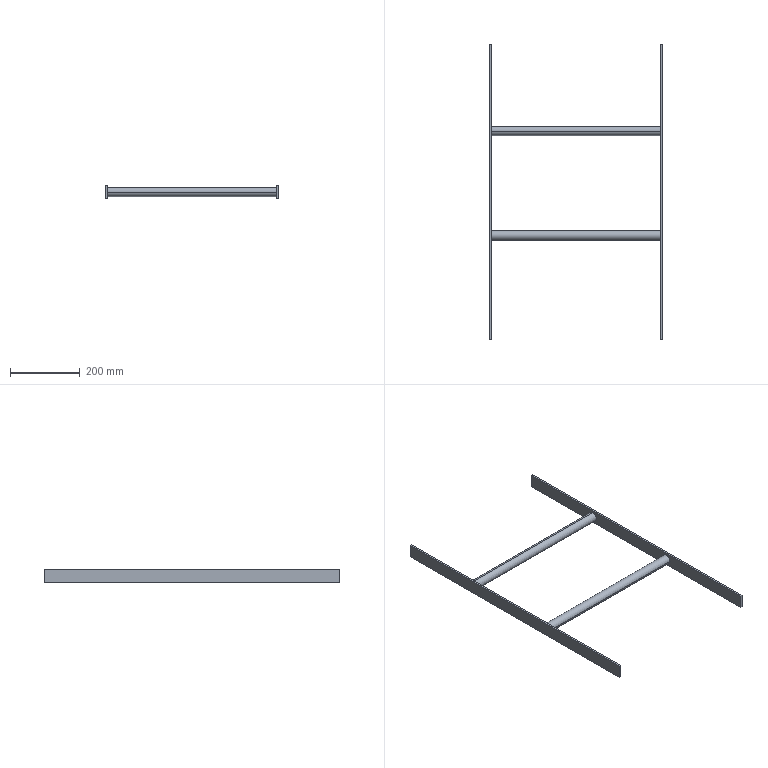Part | SolidWorks | features WeldMemberFeat 2, WeldmentFeature 1 | 4 solids | 24 faces | box 500 x 850 x 40 mm | volume 626926 mm3 | plane 16 | cylinder 8 | commonest cylinder face diameters 20.8 x4 26.8 x4
STEP:
#1=CARTESIAN_POINT('',(-250.,-425.,0.));
#2=VERTEX_POINT('',#1);
#3=CARTESIAN_POINT('',(-250.,-425.,40.));
#4=VERTEX_POINT('',#3);
#5=CARTESIAN_POINT('',(-250.,-425.,40.));
#6=DIRECTION('',(0.,0.,1.));
#7=VECTOR('',#6,1000.);
#8=LINE('',#5,#7);
#9=EDGE_CURVE('',#2,#4,#8,.T.);
#10=ORIENTED_EDGE('',*,*,#9,.T.);
#11=CARTESIAN_POINT('',(-250.,425.,40.));
#12=VERTEX_POINT('',#11);
#13=CARTESIAN_POINT('',(-250.,425.,40.));
#14=DIRECTION('',(0.,-1.,0.));
#15=VECTOR('',#14,1000.);
#16=LINE('',#13,#15);
#17=EDGE_CURVE('',#12,#4,#16,.T.);
#18=ORIENTED_EDGE('',*,*,#17,.F.);
#19=CARTESIAN_POINT('',(-250.,425.,0.));
#20=VERTEX_POINT('',#19);
#21=CARTESIAN_POINT('',(-250.,425.,40.));
#22=DIRECTION('',(0.,0.,1.));
#23=VECTOR('',#22,1000.);
#24=LINE('',#21,#23);
#25=EDGE_CURVE('',#20,#12,#24,.T.);
#26=ORIENTED_EDGE('',*,*,#25,.F.);
#27=CARTESIAN_POINT('',(-250.,425.,0.));
#28=DIRECTION('',(0.,-1.,0.));
#29=VECTOR('',#28,1000.);
#30=LINE('',#27,#29);
#31=EDGE_CURVE('',#20,#2,#30,.T.);
#32=ORIENTED_EDGE('',*,*,#31,.T.);
#33=EDGE_LOOP('',(#10,#18,#26,#32));
#34=FACE_OUTER_BOUND('',#33,.T.);
#35=CARTESIAN_POINT('',(-250.,425.,40.));
#36=DIRECTION('',(1.,0.,0.));
#37=DIRECTION('',(0.,0.,-1.));
#38=AXIS2_PLACEMENT_3D('',#35,#36,#37);
#39=PLANE('',#38);
#40=ADVANCED_FACE('',(#34),#39,.F.);
#41=CARTESIAN_POINT('',(-244.,-425.,40.));
#42=VERTEX_POINT('',#41);
#43=CARTESIAN_POINT('',(-250.,-425.,40.));
#44=DIRECTION('',(1.,0.,0.));
#45=VECTOR('',#44,1000.);
#46=LINE('',#43,#45);
#47=EDGE_CURVE('',#4,#42,#46,.T.);
#48=ORIENTED_EDGE('',*,*,#47,.T.);
#49=CARTESIAN_POINT('',(-244.,425.,40.));
#50=VERTEX_POINT('',#49);
#51=CARTESIAN_POINT('',(-244.,425.,40.));
#52=DIRECTION('',(0.,-1.,0.));
#53=VECTOR('',#52,1000.);
#54=LINE('',#51,#53);
#55=EDGE_CURVE('',#50,#42,#54,.T.);
#56=ORIENTED_EDGE('',*,*,#55,.F.);
#57=CARTESIAN_POINT('',(-250.,425.,40.));
#58=DIRECTION('',(1.,0.,0.));
#59=VECTOR('',#58,1000.);
#60=LINE('',#57,#59);
#61=EDGE_CURVE('',#12,#50,#60,.T.);
#62=ORIENTED_EDGE('',*,*,#61,.F.);
#63=ORIENTED_EDGE('',*,*,#17,.T.);
#64=EDGE_LOOP('',(#48,#56,#62,#63));
#65=FACE_OUTER_BOUND('',#64,.T.);
#66=CARTESIAN_POINT('',(-250.,425.,40.));
#67=DIRECTION('',(0.,0.,-1.));
#68=DIRECTION('',(-1.,0.,0.));
#69=AXIS2_PLACEMENT_3D('',#66,#67,#68);
#70=PLANE('',#69);
#71=ADVANCED_FACE('',(#65),#70,.F.);
#72=CARTESIAN_POINT('',(-244.,-425.,0.));
#73=VERTEX_POINT('',#72);
#74=CARTESIAN_POINT('',(-244.,-425.,0.));
#75=DIRECTION('',(0.,0.,-1.));
#76=VECTOR('',#75,1000.);
#77=LINE('',#74,#76);
#78=EDGE_CURVE('',#42,#73,#77,.T.);
#79=ORIENTED_EDGE('',*,*,#78,.T.);
#80=CARTESIAN_POINT('',(-244.,425.,0.));
#81=VERTEX_POINT('',#80);
#82=CARTESIAN_POINT('',(-244.,425.,0.));
#83=DIRECTION('',(0.,-1.,0.));
#84=VECTOR('',#83,1000.);
#85=LINE('',#82,#84);
#86=EDGE_CURVE('',#81,#73,#85,.T.);
#87=ORIENTED_EDGE('',*,*,#86,.F.);
#88=CARTESIAN_POINT('',(-244.,425.,0.));
#89=DIRECTION('',(0.,0.,-1.));
#90=VECTOR('',#89,1000.);
#91=LINE('',#88,#90);
#92=EDGE_CURVE('',#50,#81,#91,.T.);
#93=ORIENTED_EDGE('',*,*,#92,.F.);
#94=ORIENTED_EDGE('',*,*,#55,.T.);
#95=EDGE_LOOP('',(#79,#87,#93,#94));
#96=FACE_OUTER_BOUND('',#95,.T.);
#97=CARTESIAN_POINT('',(-244.,425.,0.));
#98=DIRECTION('',(-1.,0.,0.));
#99=DIRECTION('',(0.,0.,1.));
#100=AXIS2_PLACEMENT_3D('',#97,#98,#99);
#101=PLANE('',#100);
#102=ADVANCED_FACE('',(#96),#101,.F.);
#103=CARTESIAN_POINT('',(-250.,-425.,0.));
#104=DIRECTION('',(-1.,0.,0.));
#105=VECTOR('',#104,1000.);
#106=LINE('',#103,#105);
#107=EDGE_CURVE('',#73,#2,#106,.T.);
#108=ORIENTED_EDGE('',*,*,#107,.T.);
#109=ORIENTED_EDGE('',*,*,#31,.F.);
#110=CARTESIAN_POINT('',(-250.,425.,0.));
#111=DIRECTION('',(-1.,0.,0.));
#112=VECTOR('',#111,1000.);
#113=LINE('',#110,#112);
#114=EDGE_CURVE('',#81,#20,#113,.T.);
#115=ORIENTED_EDGE('',*,*,#114,.F.);
#116=ORIENTED_EDGE('',*,*,#86,.T.);
#117=EDGE_LOOP('',(#108,#109,#115,#116));
#118=FACE_OUTER_BOUND('',#117,.T.);
#119=CARTESIAN_POINT('',(-250.,425.,0.));
#120=DIRECTION('',(0.,0.,1.));
#121=DIRECTION('',(1.,0.,0.));
#122=AXIS2_PLACEMENT_3D('',#119,#120,#121);
#123=PLANE('',#122);
#124=ADVANCED_FACE('',(#118),#123,.F.);
#125=ORIENTED_EDGE('',*,*,#25,.T.);
#126=ORIENTED_EDGE('',*,*,#61,.T.);
#127=ORIENTED_EDGE('',*,*,#92,.T.);
#128=ORIENTED_EDGE('',*,*,#114,.T.);
#129=EDGE_LOOP('',(#125,#126,#127,#128));
#130=FACE_OUTER_BOUND('',#129,.T.);
#131=CARTESIAN_POINT('',(0.,425.,0.));
#132=DIRECTION('',(0.,-1.,0.));
#133=DIRECTION('',(0.,0.,-1.));
#134=AXIS2_PLACEMENT_3D('',#131,#132,#133);
#135=PLANE('',#134);
#136=ADVANCED_FACE('',(#130),#135,.F.);
#137=ORIENTED_EDGE('',*,*,#9,.F.);
#138=ORIENTED_EDGE('',*,*,#107,.F.);
#139=ORIENTED_EDGE('',*,*,#78,.F.);
#140=ORIENTED_EDGE('',*,*,#47,.F.);
#141=EDGE_LOOP('',(#137,#138,#139,#140));
#142=FACE_OUTER_BOUND('',#141,.T.);
#143=CARTESIAN_POINT('',(0.,-425.,0.));
#144=DIRECTION('',(0.,-1.,0.));
#145=DIRECTION('',(0.,0.,-1.));
#146=AXIS2_PLACEMENT_3D('',#143,#144,#145);
#147=PLANE('',#146);
#148=ADVANCED_FACE('',(#142),#147,.T.);
#149=CLOSED_SHELL('',(#40,#71,#102,#124,#136,#148));
#150=MANIFOLD_SOLID_BREP('',#149);
#151=CARTESIAN_POINT('',(250.,-425.,0.));
#152=VERTEX_POINT('',#151);
#153=CARTESIAN_POINT('',(250.,-425.,40.));
#154=VERTEX_POINT('',#153);
#155=CARTESIAN_POINT('',(250.,-425.,40.));
#156=DIRECTION('',(0.,0.,1.));
#157=VECTOR('',#156,1000.);
#158=LINE('',#155,#157);
#159=EDGE_CURVE('',#152,#154,#158,.T.);
#160=ORIENTED_EDGE('',*,*,#159,.F.);
#161=CARTESIAN_POINT('',(250.,425.,0.));
#162=VERTEX_POINT('',#161);
#163=CARTESIAN_POINT('',(250.,425.,0.));
#164=DIRECTION('',(0.,-1.,0.));
#165=VECTOR('',#164,1000.);
#166=LINE('',#163,#165);
#167=EDGE_CURVE('',#162,#152,#166,.T.);
#168=ORIENTED_EDGE('',*,*,#167,.F.);
#169=CARTESIAN_POINT('',(250.,425.,40.));
#170=VERTEX_POINT('',#169);
#171=CARTESIAN_POINT('',(250.,425.,40.));
#172=DIRECTION('',(0.,0.,1.));
#173=VECTOR('',#172,1000.);
#174=LINE('',#171,#173);
#175=EDGE_CURVE('',#162,#170,#174,.T.);
#176=ORIENTED_EDGE('',*,*,#175,.T.);
#177=CARTESIAN_POINT('',(250.,425.,40.));
#178=DIRECTION('',(0.,-1.,0.));
#179=VECTOR('',#178,1000.);
#180=LINE('',#177,#179);
#181=EDGE_CURVE('',#170,#154,#180,.T.);
#182=ORIENTED_EDGE('',*,*,#181,.T.);
#183=EDGE_LOOP('',(#160,#168,#176,#182));
#184=FACE_OUTER_BOUND('',#183,.T.);
#185=CARTESIAN_POINT('',(250.,425.,40.));
#186=DIRECTION('',(1.,0.,0.));
#187=DIRECTION('',(0.,0.,-1.));
#188=AXIS2_PLACEMENT_3D('',#185,#186,#187);
#189=PLANE('',#188);
#190=ADVANCED_FACE('',(#184),#189,.T.);
#191=CARTESIAN_POINT('',(244.,-425.,0.));
#192=VERTEX_POINT('',#191);
#193=CARTESIAN_POINT('',(250.,-425.,0.));
#194=DIRECTION('',(1.,0.,0.));
#195=VECTOR('',#194,1000.);
#196=LINE('',#193,#195);
#197=EDGE_CURVE('',#192,#152,#196,.T.);
#198=ORIENTED_EDGE('',*,*,#197,.F.);
#199=CARTESIAN_POINT('',(244.,425.,0.));
#200=VERTEX_POINT('',#199);
#201=CARTESIAN_POINT('',(244.,425.,0.));
#202=DIRECTION('',(0.,-1.,0.));
#203=VECTOR('',#202,1000.);
#204=LINE('',#201,#203);
#205=EDGE_CURVE('',#200,#192,#204,.T.);
#206=ORIENTED_EDGE('',*,*,#205,.F.);
#207=CARTESIAN_POINT('',(250.,425.,0.));
#208=DIRECTION('',(1.,0.,0.));
#209=VECTOR('',#208,1000.);
#210=LINE('',#207,#209);
#211=EDGE_CURVE('',#200,#162,#210,.T.);
#212=ORIENTED_EDGE('',*,*,#211,.T.);
#213=ORIENTED_EDGE('',*,*,#167,.T.);
#214=EDGE_LOOP('',(#198,#206,#212,#213));
#215=FACE_OUTER_BOUND('',#214,.T.);
#216=CARTESIAN_POINT('',(250.,425.,0.));
#217=DIRECTION('',(0.,0.,-1.));
#218=DIRECTION('',(-1.,0.,0.));
#219=AXIS2_PLACEMENT_3D('',#216,#217,#218);
#220=PLANE('',#219);
#221=ADVANCED_FACE('',(#215),#220,.T.);
#222=CARTESIAN_POINT('',(244.,-425.,40.));
#223=VERTEX_POINT('',#222);
#224=CARTESIAN_POINT('',(244.,-425.,0.));
#225=DIRECTION('',(0.,0.,-1.));
#226=VECTOR('',#225,1000.);
#227=LINE('',#224,#226);
#228=EDGE_CURVE('',#223,#192,#227,.T.);
#229=ORIENTED_EDGE('',*,*,#228,.F.);
#230=CARTESIAN_POINT('',(244.,425.,40.));
#231=VERTEX_POINT('',#230);
#232=CARTESIAN_POINT('',(244.,425.,40.));
#233=DIRECTION('',(0.,-1.,0.));
#234=VECTOR('',#233,1000.);
#235=LINE('',#232,#234);
#236=EDGE_CURVE('',#231,#223,#235,.T.);
#237=ORIENTED_EDGE('',*,*,#236,.F.);
#238=CARTESIAN_POINT('',(244.,425.,0.));
#239=DIRECTION('',(0.,0.,-1.));
#240=VECTOR('',#239,1000.);
#241=LINE('',#238,#240);
#242=EDGE_CURVE('',#231,#200,#241,.T.);
#243=ORIENTED_EDGE('',*,*,#242,.T.);
#244=ORIENTED_EDGE('',*,*,#205,.T.);
#245=EDGE_LOOP('',(#229,#237,#243,#244));
#246=FACE_OUTER_BOUND('',#245,.T.);
#247=CARTESIAN_POINT('',(244.,425.,0.));
#248=DIRECTION('',(-1.,0.,0.));
#249=DIRECTION('',(0.,0.,1.));
#250=AXIS2_PLACEMENT_3D('',#247,#248,#249);
#251=PLANE('',#250);
#252=ADVANCED_FACE('',(#246),#251,.T.);
#253=CARTESIAN_POINT('',(250.,-425.,40.));
#254=DIRECTION('',(-1.,0.,0.));
#255=VECTOR('',#254,1000.);
#256=LINE('',#253,#255);
#257=EDGE_CURVE('',#154,#223,#256,.T.);
#258=ORIENTED_EDGE('',*,*,#257,.F.);
#259=ORIENTED_EDGE('',*,*,#181,.F.);
#260=CARTESIAN_POINT('',(250.,425.,40.));
#261=DIRECTION('',(-1.,0.,0.));
#262=VECTOR('',#261,1000.);
#263=LINE('',#260,#262);
#264=EDGE_CURVE('',#170,#231,#263,.T.);
#265=ORIENTED_EDGE('',*,*,#264,.T.);
#266=ORIENTED_EDGE('',*,*,#236,.T.);
#267=EDGE_LOOP('',(#258,#259,#265,#266));
#268=FACE_OUTER_BOUND('',#267,.T.);
#269=CARTESIAN_POINT('',(250.,425.,40.));
#270=DIRECTION('',(0.,0.,1.));
#271=DIRECTION('',(1.,0.,0.));
#272=AXIS2_PLACEMENT_3D('',#269,#270,#271);
#273=PLANE('',#272);
#274=ADVANCED_FACE('',(#268),#273,.T.);
#275=ORIENTED_EDGE('',*,*,#175,.F.);
#276=ORIENTED_EDGE('',*,*,#211,.F.);
#277=ORIENTED_EDGE('',*,*,#242,.F.);
#278=ORIENTED_EDGE('',*,*,#264,.F.);
#279=EDGE_LOOP('',(#275,#276,#277,#278));
#280=FACE_OUTER_BOUND('',#279,.T.);
#281=CARTESIAN_POINT('',(0.,425.,0.));
#282=DIRECTION('',(0.,1.,0.));
#283=DIRECTION('',(0.,0.,-1.));
#284=AXIS2_PLACEMENT_3D('',#281,#282,#283);
#285=PLANE('',#284);
#286=ADVANCED_FACE('',(#280),#285,.T.);
#287=ORIENTED_EDGE('',*,*,#159,.T.);
#288=ORIENTED_EDGE('',*,*,#257,.T.);
#289=ORIENTED_EDGE('',*,*,#228,.T.);
#290=ORIENTED_EDGE('',*,*,#197,.T.);
#291=EDGE_LOOP('',(#287,#288,#289,#290));
#292=FACE_OUTER_BOUND('',#291,.T.);
#293=CARTESIAN_POINT('',(0.,-425.,0.));
#294=DIRECTION('',(0.,1.,0.));
#295=DIRECTION('',(0.,0.,-1.));
#296=AXIS2_PLACEMENT_3D('',#293,#294,#295);
#297=PLANE('',#296);
#298=ADVANCED_FACE('',(#292),#297,.F.);
#299=CLOSED_SHELL('',(#190,#221,#252,#274,#286,#298));
#300=MANIFOLD_SOLID_BREP('',#299);
#301=CARTESIAN_POINT('',(244.,175.,6.6));
#302=VERTEX_POINT('',#301);
#303=CARTESIAN_POINT('',(244.,175.,33.4));
#304=VERTEX_POINT('',#303);
#305=CARTESIAN_POINT('',(244.,175.,20.));
#306=DIRECTION('',(1.,0.,0.));
#307=DIRECTION('',(0.,0.,-1.));
#308=AXIS2_PLACEMENT_3D('',#305,#306,#307);
#309=CIRCLE('',#308,13.4);
#310=EDGE_CURVE('',#302,#304,#309,.T.);
#311=ORIENTED_EDGE('',*,*,#310,.F.);
#312=CARTESIAN_POINT('',(-244.,175.,6.6));
#313=VERTEX_POINT('',#312);
#314=CARTESIAN_POINT('',(244.,175.,6.6));
#315=DIRECTION('',(-1.,0.,0.));
#316=VECTOR('',#315,1000.);
#317=LINE('',#314,#316);
#318=EDGE_CURVE('',#302,#313,#317,.T.);
#319=ORIENTED_EDGE('',*,*,#318,.T.);
#320=CARTESIAN_POINT('',(-244.,175.,33.4));
#321=VERTEX_POINT('',#320);
#322=CARTESIAN_POINT('',(-244.,175.,20.));
#323=DIRECTION('',(1.,0.,0.));
#324=DIRECTION('',(0.,0.,-1.));
#325=AXIS2_PLACEMENT_3D('',#322,#323,#324);
#326=CIRCLE('',#325,13.4);
#327=EDGE_CURVE('',#313,#321,#326,.T.);
#328=ORIENTED_EDGE('',*,*,#327,.T.);
#329=CARTESIAN_POINT('',(244.,175.,33.4));
#330=DIRECTION('',(-1.,0.,0.));
#331=VECTOR('',#330,1000.);
#332=LINE('',#329,#331);
#333=EDGE_CURVE('',#304,#321,#332,.T.);
#334=ORIENTED_EDGE('',*,*,#333,.F.);
#335=EDGE_LOOP('',(#311,#319,#328,#334));
#336=FACE_OUTER_BOUND('',#335,.T.);
#337=CARTESIAN_POINT('',(244.,175.,20.));
#338=DIRECTION('',(-1.,0.,0.));
#339=DIRECTION('',(0.,0.,1.));
#340=AXIS2_PLACEMENT_3D('',#337,#338,#339);
#341=CYLINDRICAL_SURFACE('',#340,13.4);
#342=ADVANCED_FACE('',(#336),#341,.T.);
#343=CARTESIAN_POINT('',(244.,175.,30.4));
#344=VERTEX_POINT('',#343);
#345=CARTESIAN_POINT('',(244.,175.,9.6));
#346=VERTEX_POINT('',#345);
#347=CARTESIAN_POINT('',(244.,175.,20.));
#348=DIRECTION('',(1.,0.,0.));
#349=DIRECTION('',(0.,0.,-1.));
#350=AXIS2_PLACEMENT_3D('',#347,#348,#349);
#351=CIRCLE('',#350,10.4);
#352=EDGE_CURVE('',#344,#346,#351,.T.);
#353=ORIENTED_EDGE('',*,*,#352,.T.);
#354=CARTESIAN_POINT('',(-244.,175.,9.6));
#355=VERTEX_POINT('',#354);
#356=CARTESIAN_POINT('',(244.,175.,9.6));
#357=DIRECTION('',(-1.,0.,0.));
#358=VECTOR('',#357,1000.);
#359=LINE('',#356,#358);
#360=EDGE_CURVE('',#346,#355,#359,.T.);
#361=ORIENTED_EDGE('',*,*,#360,.T.);
#362=CARTESIAN_POINT('',(-244.,175.,30.4));
#363=VERTEX_POINT('',#362);
#364=CARTESIAN_POINT('',(-244.,175.,20.));
#365=DIRECTION('',(1.,0.,0.));
#366=DIRECTION('',(0.,0.,-1.));
#367=AXIS2_PLACEMENT_3D('',#364,#365,#366);
#368=CIRCLE('',#367,10.4);
#369=EDGE_CURVE('',#363,#355,#368,.T.);
#370=ORIENTED_EDGE('',*,*,#369,.F.);
#371=CARTESIAN_POINT('',(244.,175.,30.4));
#372=DIRECTION('',(-1.,0.,0.));
#373=VECTOR('',#372,1000.);
#374=LINE('',#371,#373);
#375=EDGE_CURVE('',#344,#363,#374,.T.);
#376=ORIENTED_EDGE('',*,*,#375,.F.);
#377=EDGE_LOOP('',(#353,#361,#370,#376));
#378=FACE_OUTER_BOUND('',#377,.T.);
#379=CARTESIAN_POINT('',(244.,175.,20.));
#380=DIRECTION('',(-1.,0.,0.));
#381=DIRECTION('',(0.,0.,1.));
#382=AXIS2_PLACEMENT_3D('',#379,#380,#381);
#383=CYLINDRICAL_SURFACE('',#382,10.4);
#384=ADVANCED_FACE('',(#378),#383,.F.);
#385=ORIENTED_EDGE('',*,*,#360,.F.);
#386=CARTESIAN_POINT('',(244.,175.,20.));
#387=DIRECTION('',(1.,0.,0.));
#388=DIRECTION('',(0.,0.,-1.));
#389=AXIS2_PLACEMENT_3D('',#386,#387,#388);
#390=CIRCLE('',#389,10.4);
#391=EDGE_CURVE('',#346,#344,#390,.T.);
#392=ORIENTED_EDGE('',*,*,#391,.T.);
#393=ORIENTED_EDGE('',*,*,#375,.T.);
#394=CARTESIAN_POINT('',(-244.,175.,20.));
#395=DIRECTION('',(1.,0.,0.));
#396=DIRECTION('',(0.,0.,-1.));
#397=AXIS2_PLACEMENT_3D('',#394,#395,#396);
#398=CIRCLE('',#397,10.4);
#399=EDGE_CURVE('',#355,#363,#398,.T.);
#400=ORIENTED_EDGE('',*,*,#399,.F.);
#401=EDGE_LOOP('',(#385,#392,#393,#400));
#402=FACE_OUTER_BOUND('',#401,.T.);
#403=CARTESIAN_POINT('',(244.,175.,20.));
#404=DIRECTION('',(-1.,0.,0.));
#405=DIRECTION('',(0.,0.,1.));
#406=AXIS2_PLACEMENT_3D('',#403,#404,#405);
#407=CYLINDRICAL_SURFACE('',#406,10.4);
#408=ADVANCED_FACE('',(#402),#407,.F.);
#409=ORIENTED_EDGE('',*,*,#318,.F.);
#410=CARTESIAN_POINT('',(244.,175.,20.));
#411=DIRECTION('',(1.,0.,0.));
#412=DIRECTION('',(0.,0.,-1.));
#413=AXIS2_PLACEMENT_3D('',#410,#411,#412);
#414=CIRCLE('',#413,13.4);
#415=EDGE_CURVE('',#304,#302,#414,.T.);
#416=ORIENTED_EDGE('',*,*,#415,.F.);
#417=ORIENTED_EDGE('',*,*,#333,.T.);
#418=CARTESIAN_POINT('',(-244.,175.,20.));
#419=DIRECTION('',(1.,0.,0.));
#420=DIRECTION('',(0.,0.,-1.));
#421=AXIS2_PLACEMENT_3D('',#418,#419,#420);
#422=CIRCLE('',#421,13.4);
#423=EDGE_CURVE('',#321,#313,#422,.T.);
#424=ORIENTED_EDGE('',*,*,#423,.T.);
#425=EDGE_LOOP('',(#409,#416,#417,#424));
#426=FACE_OUTER_BOUND('',#425,.T.);
#427=CARTESIAN_POINT('',(244.,175.,20.));
#428=DIRECTION('',(-1.,0.,0.));
#429=DIRECTION('',(0.,0.,1.));
#430=AXIS2_PLACEMENT_3D('',#427,#428,#429);
#431=CYLINDRICAL_SURFACE('',#430,13.4);
#432=ADVANCED_FACE('',(#426),#431,.T.);
#433=ORIENTED_EDGE('',*,*,#352,.F.);
#434=ORIENTED_EDGE('',*,*,#391,.F.);
#435=EDGE_LOOP('',(#433,#434));
#436=FACE_BOUND('',#435,.T.);
#437=ORIENTED_EDGE('',*,*,#415,.T.);
#438=ORIENTED_EDGE('',*,*,#310,.T.);
#439=EDGE_LOOP('',(#437,#438));
#440=FACE_OUTER_BOUND('',#439,.T.);
#441=CARTESIAN_POINT('',(244.,175.,20.));
#442=DIRECTION('',(1.,0.,0.));
#443=DIRECTION('',(0.,0.,-1.));
#444=AXIS2_PLACEMENT_3D('',#441,#442,#443);
#445=PLANE('',#444);
#446=ADVANCED_FACE('',(#436,#440),#445,.T.);
#447=ORIENTED_EDGE('',*,*,#369,.T.);
#448=ORIENTED_EDGE('',*,*,#399,.T.);
#449=EDGE_LOOP('',(#447,#448));
#450=FACE_BOUND('',#449,.T.);
#451=ORIENTED_EDGE('',*,*,#423,.F.);
#452=ORIENTED_EDGE('',*,*,#327,.F.);
#453=EDGE_LOOP('',(#451,#452));
#454=FACE_OUTER_BOUND('',#453,.T.);
#455=CARTESIAN_POINT('',(-244.,175.,20.));
#456=DIRECTION('',(1.,0.,0.));
#457=DIRECTION('',(0.,0.,-1.));
#458=AXIS2_PLACEMENT_3D('',#455,#456,#457);
#459=PLANE('',#458);
#460=ADVANCED_FACE('',(#450,#454),#459,.F.);
#461=CLOSED_SHELL('',(#342,#384,#408,#432,#446,#460));
#462=MANIFOLD_SOLID_BREP('',#461);
#463=CARTESIAN_POINT('',(244.,-111.6,20.));
#464=VERTEX_POINT('',#463);
#465=CARTESIAN_POINT('',(244.,-138.4,20.));
#466=VERTEX_POINT('',#465);
#467=CARTESIAN_POINT('',(244.,-125.,20.));
#468=DIRECTION('',(1.,0.,0.));
#469=DIRECTION('',(0.,0.,-1.));
#470=AXIS2_PLACEMENT_3D('',#467,#468,#469);
#471=CIRCLE('',#470,13.4);
#472=EDGE_CURVE('',#464,#466,#471,.T.);
#473=ORIENTED_EDGE('',*,*,#472,.F.);
#474=CARTESIAN_POINT('',(-244.,-111.6,20.));
#475=VERTEX_POINT('',#474);
#476=CARTESIAN_POINT('',(244.,-111.6,20.));
#477=DIRECTION('',(-1.,0.,0.));
#478=VECTOR('',#477,1000.);
#479=LINE('',#476,#478);
#480=EDGE_CURVE('',#464,#475,#479,.T.);
#481=ORIENTED_EDGE('',*,*,#480,.T.);
#482=CARTESIAN_POINT('',(-244.,-138.4,20.));
#483=VERTEX_POINT('',#482);
#484=CARTESIAN_POINT('',(-244.,-125.,20.));
#485=DIRECTION('',(1.,0.,0.));
#486=DIRECTION('',(0.,0.,-1.));
#487=AXIS2_PLACEMENT_3D('',#484,#485,#486);
#488=CIRCLE('',#487,13.4);
#489=EDGE_CURVE('',#475,#483,#488,.T.);
#490=ORIENTED_EDGE('',*,*,#489,.T.);
#491=CARTESIAN_POINT('',(244.,-138.4,20.));
#492=DIRECTION('',(-1.,0.,0.));
#493=VECTOR('',#492,1000.);
#494=LINE('',#491,#493);
#495=EDGE_CURVE('',#466,#483,#494,.T.);
#496=ORIENTED_EDGE('',*,*,#495,.F.);
#497=EDGE_LOOP('',(#473,#481,#490,#496));
#498=FACE_OUTER_BOUND('',#497,.T.);
#499=CARTESIAN_POINT('',(244.,-125.,20.));
#500=DIRECTION('',(-1.,0.,0.));
#501=DIRECTION('',(0.,-1.,0.));
#502=AXIS2_PLACEMENT_3D('',#499,#500,#501);
#503=CYLINDRICAL_SURFACE('',#502,13.4);
#504=ADVANCED_FACE('',(#498),#503,.T.);
#505=CARTESIAN_POINT('',(244.,-135.4,20.));
#506=VERTEX_POINT('',#505);
#507=CARTESIAN_POINT('',(244.,-114.6,20.));
#508=VERTEX_POINT('',#507);
#509=CARTESIAN_POINT('',(244.,-125.,20.));
#510=DIRECTION('',(1.,0.,0.));
#511=DIRECTION('',(0.,0.,-1.));
#512=AXIS2_PLACEMENT_3D('',#509,#510,#511);
#513=CIRCLE('',#512,10.4);
#514=EDGE_CURVE('',#506,#508,#513,.T.);
#515=ORIENTED_EDGE('',*,*,#514,.T.);
#516=CARTESIAN_POINT('',(-244.,-114.6,20.));
#517=VERTEX_POINT('',#516);
#518=CARTESIAN_POINT('',(244.,-114.6,20.));
#519=DIRECTION('',(-1.,0.,0.));
#520=VECTOR('',#519,1000.);
#521=LINE('',#518,#520);
#522=EDGE_CURVE('',#508,#517,#521,.T.);
#523=ORIENTED_EDGE('',*,*,#522,.T.);
#524=CARTESIAN_POINT('',(-244.,-135.4,20.));
#525=VERTEX_POINT('',#524);
#526=CARTESIAN_POINT('',(-244.,-125.,20.));
#527=DIRECTION('',(1.,0.,0.));
#528=DIRECTION('',(0.,0.,-1.));
#529=AXIS2_PLACEMENT_3D('',#526,#527,#528);
#530=CIRCLE('',#529,10.4);
#531=EDGE_CURVE('',#525,#517,#530,.T.);
#532=ORIENTED_EDGE('',*,*,#531,.F.);
#533=CARTESIAN_POINT('',(244.,-135.4,20.));
#534=DIRECTION('',(-1.,0.,0.));
#535=VECTOR('',#534,1000.);
#536=LINE('',#533,#535);
#537=EDGE_CURVE('',#506,#525,#536,.T.);
#538=ORIENTED_EDGE('',*,*,#537,.F.);
#539=EDGE_LOOP('',(#515,#523,#532,#538));
#540=FACE_OUTER_BOUND('',#539,.T.);
#541=CARTESIAN_POINT('',(244.,-125.,20.));
#542=DIRECTION('',(-1.,0.,0.));
#543=DIRECTION('',(0.,-1.,0.));
#544=AXIS2_PLACEMENT_3D('',#541,#542,#543);
#545=CYLINDRICAL_SURFACE('',#544,10.4);
#546=ADVANCED_FACE('',(#540),#545,.F.);
#547=ORIENTED_EDGE('',*,*,#522,.F.);
#548=CARTESIAN_POINT('',(244.,-125.,20.));
#549=DIRECTION('',(1.,0.,0.));
#550=DIRECTION('',(0.,0.,-1.));
#551=AXIS2_PLACEMENT_3D('',#548,#549,#550);
#552=CIRCLE('',#551,10.4);
#553=EDGE_CURVE('',#508,#506,#552,.T.);
#554=ORIENTED_EDGE('',*,*,#553,.T.);
#555=ORIENTED_EDGE('',*,*,#537,.T.);
#556=CARTESIAN_POINT('',(-244.,-125.,20.));
#557=DIRECTION('',(1.,0.,0.));
#558=DIRECTION('',(0.,0.,-1.));
#559=AXIS2_PLACEMENT_3D('',#556,#557,#558);
#560=CIRCLE('',#559,10.4);
#561=EDGE_CURVE('',#517,#525,#560,.T.);
#562=ORIENTED_EDGE('',*,*,#561,.F.);
#563=EDGE_LOOP('',(#547,#554,#555,#562));
#564=FACE_OUTER_BOUND('',#563,.T.);
#565=CARTESIAN_POINT('',(244.,-125.,20.));
#566=DIRECTION('',(-1.,0.,0.));
#567=DIRECTION('',(0.,-1.,0.));
#568=AXIS2_PLACEMENT_3D('',#565,#566,#567);
#569=CYLINDRICAL_SURFACE('',#568,10.4);
#570=ADVANCED_FACE('',(#564),#569,.F.);
#571=ORIENTED_EDGE('',*,*,#480,.F.);
#572=CARTESIAN_POINT('',(244.,-125.,20.));
#573=DIRECTION('',(1.,0.,0.));
#574=DIRECTION('',(0.,0.,-1.));
#575=AXIS2_PLACEMENT_3D('',#572,#573,#574);
#576=CIRCLE('',#575,13.4);
#577=EDGE_CURVE('',#466,#464,#576,.T.);
#578=ORIENTED_EDGE('',*,*,#577,.F.);
#579=ORIENTED_EDGE('',*,*,#495,.T.);
#580=CARTESIAN_POINT('',(-244.,-125.,20.));
#581=DIRECTION('',(1.,0.,0.));
#582=DIRECTION('',(0.,0.,-1.));
#583=AXIS2_PLACEMENT_3D('',#580,#581,#582);
#584=CIRCLE('',#583,13.4);
#585=EDGE_CURVE('',#483,#475,#584,.T.);
#586=ORIENTED_EDGE('',*,*,#585,.T.);
#587=EDGE_LOOP('',(#571,#578,#579,#586));
#588=FACE_OUTER_BOUND('',#587,.T.);
#589=CARTESIAN_POINT('',(244.,-125.,20.));
#590=DIRECTION('',(-1.,0.,0.));
#591=DIRECTION('',(0.,-1.,0.));
#592=AXIS2_PLACEMENT_3D('',#589,#590,#591);
#593=CYLINDRICAL_SURFACE('',#592,13.4);
#594=ADVANCED_FACE('',(#588),#593,.T.);
#595=ORIENTED_EDGE('',*,*,#514,.F.);
#596=ORIENTED_EDGE('',*,*,#553,.F.);
#597=EDGE_LOOP('',(#595,#596));
#598=FACE_BOUND('',#597,.T.);
#599=ORIENTED_EDGE('',*,*,#577,.T.);
#600=ORIENTED_EDGE('',*,*,#472,.T.);
#601=EDGE_LOOP('',(#599,#600));
#602=FACE_OUTER_BOUND('',#601,.T.);
#603=CARTESIAN_POINT('',(244.,-125.,20.));
#604=DIRECTION('',(1.,0.,0.));
#605=DIRECTION('',(0.,0.,-1.));
#606=AXIS2_PLACEMENT_3D('',#603,#604,#605);
#607=PLANE('',#606);
#608=ADVANCED_FACE('',(#598,#602),#607,.T.);
#609=ORIENTED_EDGE('',*,*,#531,.T.);
#610=ORIENTED_EDGE('',*,*,#561,.T.);
#611=EDGE_LOOP('',(#609,#610));
#612=FACE_BOUND('',#611,.T.);
#613=ORIENTED_EDGE('',*,*,#585,.F.);
#614=ORIENTED_EDGE('',*,*,#489,.F.);
#615=EDGE_LOOP('',(#613,#614));
#616=FACE_OUTER_BOUND('',#615,.T.);
#617=CARTESIAN_POINT('',(-244.,-125.,20.));
#618=DIRECTION('',(1.,0.,0.));
#619=DIRECTION('',(0.,0.,-1.));
#620=AXIS2_PLACEMENT_3D('',#617,#618,#619);
#621=PLANE('',#620);
#622=ADVANCED_FACE('',(#612,#616),#621,.F.);
#623=CLOSED_SHELL('',(#504,#546,#570,#594,#608,#622));
#624=MANIFOLD_SOLID_BREP('',#623);
#625=CARTESIAN_POINT('',(0.,0.,0.));
#626=DIRECTION('',(0.,0.,1.));
#627=DIRECTION('',(1.,0.,0.));
#628=AXIS2_PLACEMENT_3D('',#625,#626,#627);
#629=(LENGTH_UNIT()NAMED_UNIT(*)SI_UNIT(.MILLI.,.METRE.));
#630=UNCERTAINTY_MEASURE_WITH_UNIT(LENGTH_MEASURE(0.00001),#629,'','');
#631=(NAMED_UNIT(*)PLANE_ANGLE_UNIT()SI_UNIT($,.RADIAN.));
#632=(NAMED_UNIT(*)SI_UNIT($,.STERADIAN.)SOLID_ANGLE_UNIT());
#633=(GEOMETRIC_REPRESENTATION_CONTEXT(3)GLOBAL_UNCERTAINTY_ASSIGNED_CONTEXT((#630))GLOBAL_UNIT_ASSIGNED_CONTEXT((#629,#631,#632))REPRESENTATION_CONTEXT('',''));
#634=ADVANCED_BREP_SHAPE_REPRESENTATION('',(#150,#300,#462,#624,#628),#633);